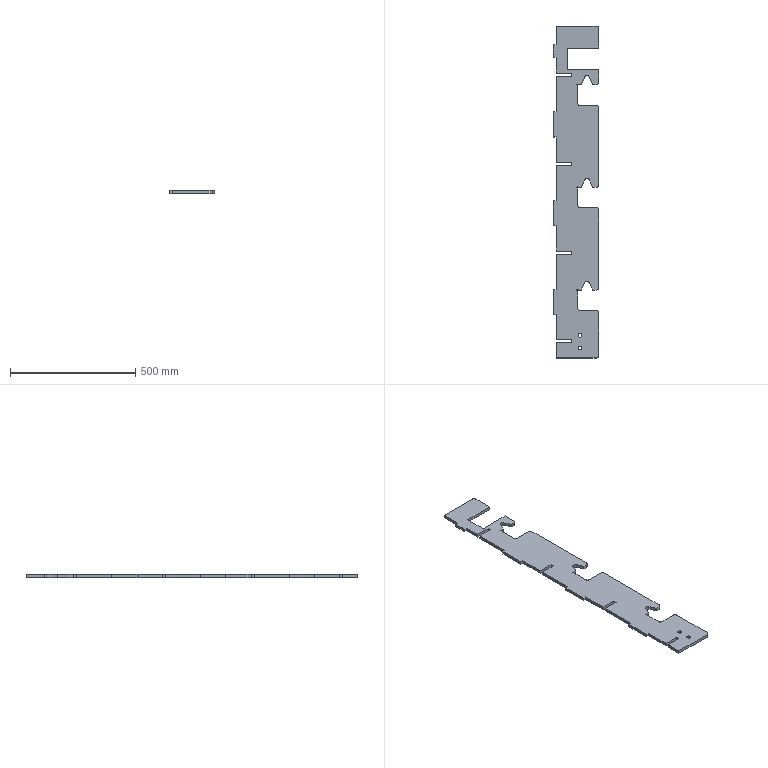Part | SolidWorks | features Fillet 2, FlatPattern 1, SMBaseFlange 1, SheetMetal 1 | 1 solid | 87 faces | box 180 x 1325 x 12 mm | volume 2282153 mm3 | plane 63 | cylinder 24 | commonest cylinder face diameters 20 x14 5 x6 15 x4